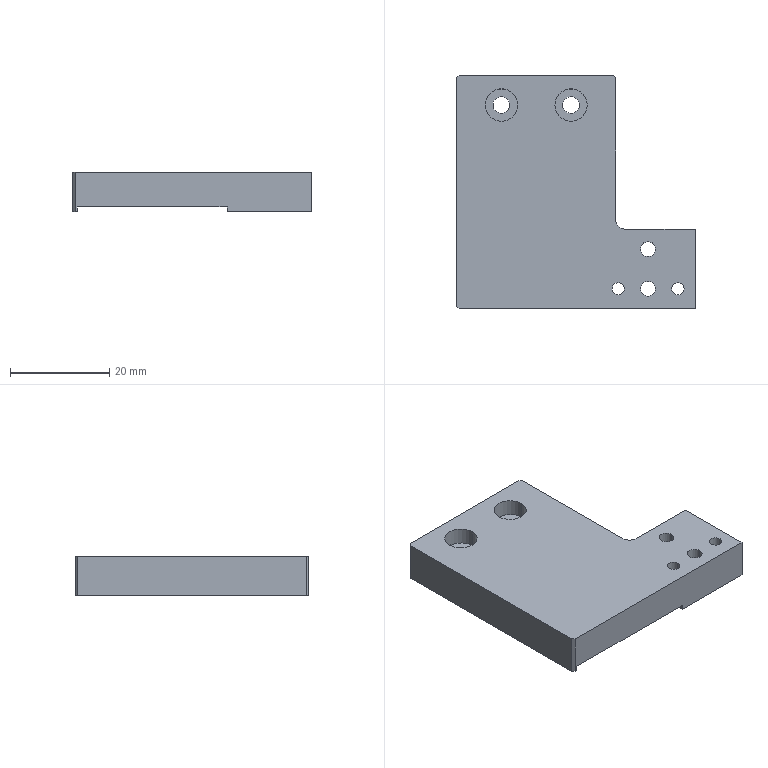Part | STEP file | 11-FG-E03411 | 1 solid | 34 faces | box 48 x 47 x 8 mm | volume 12187 mm3 | cylinder 17 | plane 17 | commonest cylinder face diameters 2.5 x4 3 x4 3.4 x4 6.5 x4 4 x1
STEP:
#1=CARTESIAN_POINT('',(21.005,-11.495,0.));
#2=VERTEX_POINT('',#1);
#3=CARTESIAN_POINT('',(24.005,-11.495,0.));
#4=VERTEX_POINT('',#3);
#5=CARTESIAN_POINT('',(22.505,-11.495,0.));
#6=DIRECTION('',(0.,0.,1.));
#7=DIRECTION('',(1.,0.,0.));
#8=AXIS2_PLACEMENT_3D('',#5,#6,#7);
#9=CIRCLE('',#8,1.5);
#10=EDGE_CURVE('',#2,#4,#9,.T.);
#11=ORIENTED_EDGE('',*,*,#10,.F.);
#12=CARTESIAN_POINT('',(21.005,-11.495,8.));
#13=VERTEX_POINT('',#12);
#14=CARTESIAN_POINT('',(21.005,-11.495,8.));
#15=DIRECTION('',(0.,0.,1.));
#16=VECTOR('',#15,1000.);
#17=LINE('',#14,#16);
#18=EDGE_CURVE('',#2,#13,#17,.T.);
#19=ORIENTED_EDGE('',*,*,#18,.T.);
#20=CARTESIAN_POINT('',(24.005,-11.495,8.));
#21=VERTEX_POINT('',#20);
#22=CARTESIAN_POINT('',(22.505,-11.495,8.));
#23=DIRECTION('',(0.,0.,1.));
#24=DIRECTION('',(1.,0.,0.));
#25=AXIS2_PLACEMENT_3D('',#22,#23,#24);
#26=CIRCLE('',#25,1.5);
#27=EDGE_CURVE('',#13,#21,#26,.T.);
#28=ORIENTED_EDGE('',*,*,#27,.T.);
#29=CARTESIAN_POINT('',(24.005,-11.495,8.));
#30=DIRECTION('',(0.,0.,1.));
#31=VECTOR('',#30,1000.);
#32=LINE('',#29,#31);
#33=EDGE_CURVE('',#4,#21,#32,.T.);
#34=ORIENTED_EDGE('',*,*,#33,.F.);
#35=EDGE_LOOP('',(#11,#19,#28,#34));
#36=FACE_OUTER_BOUND('',#35,.T.);
#37=CARTESIAN_POINT('',(22.505,-11.495,8.));
#38=DIRECTION('',(0.,0.,1.));
#39=DIRECTION('',(1.,0.,0.));
#40=AXIS2_PLACEMENT_3D('',#37,#38,#39);
#41=CYLINDRICAL_SURFACE('',#40,1.5);
#42=ADVANCED_FACE('',(#36),#41,.F.);
#43=CARTESIAN_POINT('',(21.005,-19.495,0.));
#44=VERTEX_POINT('',#43);
#45=CARTESIAN_POINT('',(24.005,-19.495,0.));
#46=VERTEX_POINT('',#45);
#47=CARTESIAN_POINT('',(22.505,-19.495,0.));
#48=DIRECTION('',(0.,0.,1.));
#49=DIRECTION('',(1.,0.,0.));
#50=AXIS2_PLACEMENT_3D('',#47,#48,#49);
#51=CIRCLE('',#50,1.5);
#52=EDGE_CURVE('',#44,#46,#51,.T.);
#53=ORIENTED_EDGE('',*,*,#52,.F.);
#54=CARTESIAN_POINT('',(21.005,-19.495,8.));
#55=VERTEX_POINT('',#54);
#56=CARTESIAN_POINT('',(21.005,-19.495,8.));
#57=DIRECTION('',(0.,0.,1.));
#58=VECTOR('',#57,1000.);
#59=LINE('',#56,#58);
#60=EDGE_CURVE('',#44,#55,#59,.T.);
#61=ORIENTED_EDGE('',*,*,#60,.T.);
#62=CARTESIAN_POINT('',(24.005,-19.495,8.));
#63=VERTEX_POINT('',#62);
#64=CARTESIAN_POINT('',(22.505,-19.495,8.));
#65=DIRECTION('',(0.,0.,1.));
#66=DIRECTION('',(1.,0.,0.));
#67=AXIS2_PLACEMENT_3D('',#64,#65,#66);
#68=CIRCLE('',#67,1.5);
#69=EDGE_CURVE('',#55,#63,#68,.T.);
#70=ORIENTED_EDGE('',*,*,#69,.T.);
#71=CARTESIAN_POINT('',(24.005,-19.495,8.));
#72=DIRECTION('',(0.,0.,1.));
#73=VECTOR('',#72,1000.);
#74=LINE('',#71,#73);
#75=EDGE_CURVE('',#46,#63,#74,.T.);
#76=ORIENTED_EDGE('',*,*,#75,.F.);
#77=EDGE_LOOP('',(#53,#61,#70,#76));
#78=FACE_OUTER_BOUND('',#77,.T.);
#79=CARTESIAN_POINT('',(22.505,-19.495,8.));
#80=DIRECTION('',(0.,0.,1.));
#81=DIRECTION('',(1.,0.,0.));
#82=AXIS2_PLACEMENT_3D('',#79,#80,#81);
#83=CYLINDRICAL_SURFACE('',#82,1.5);
#84=ADVANCED_FACE('',(#78),#83,.F.);
#85=CARTESIAN_POINT('',(27.255,-19.495,0.));
#86=VERTEX_POINT('',#85);
#87=CARTESIAN_POINT('',(29.755,-19.495,0.));
#88=VERTEX_POINT('',#87);
#89=CARTESIAN_POINT('',(28.505,-19.495,0.));
#90=DIRECTION('',(0.,0.,1.));
#91=DIRECTION('',(1.,0.,0.));
#92=AXIS2_PLACEMENT_3D('',#89,#90,#91);
#93=CIRCLE('',#92,1.25);
#94=EDGE_CURVE('',#86,#88,#93,.T.);
#95=ORIENTED_EDGE('',*,*,#94,.F.);
#96=CARTESIAN_POINT('',(27.255,-19.495,8.));
#97=VERTEX_POINT('',#96);
#98=CARTESIAN_POINT('',(27.255,-19.495,8.));
#99=DIRECTION('',(0.,0.,1.));
#100=VECTOR('',#99,1000.);
#101=LINE('',#98,#100);
#102=EDGE_CURVE('',#86,#97,#101,.T.);
#103=ORIENTED_EDGE('',*,*,#102,.T.);
#104=CARTESIAN_POINT('',(29.755,-19.495,8.));
#105=VERTEX_POINT('',#104);
#106=CARTESIAN_POINT('',(28.505,-19.495,8.));
#107=DIRECTION('',(0.,0.,1.));
#108=DIRECTION('',(1.,0.,0.));
#109=AXIS2_PLACEMENT_3D('',#106,#107,#108);
#110=CIRCLE('',#109,1.25);
#111=EDGE_CURVE('',#97,#105,#110,.T.);
#112=ORIENTED_EDGE('',*,*,#111,.T.);
#113=CARTESIAN_POINT('',(29.755,-19.495,8.));
#114=DIRECTION('',(0.,0.,1.));
#115=VECTOR('',#114,1000.);
#116=LINE('',#113,#115);
#117=EDGE_CURVE('',#88,#105,#116,.T.);
#118=ORIENTED_EDGE('',*,*,#117,.F.);
#119=EDGE_LOOP('',(#95,#103,#112,#118));
#120=FACE_OUTER_BOUND('',#119,.T.);
#121=CARTESIAN_POINT('',(28.505,-19.495,8.));
#122=DIRECTION('',(0.,0.,1.));
#123=DIRECTION('',(1.,0.,0.));
#124=AXIS2_PLACEMENT_3D('',#121,#122,#123);
#125=CYLINDRICAL_SURFACE('',#124,1.25);
#126=ADVANCED_FACE('',(#120),#125,.F.);
#127=CARTESIAN_POINT('',(15.255,-19.495,0.));
#128=VERTEX_POINT('',#127);
#129=CARTESIAN_POINT('',(17.755,-19.495,0.));
#130=VERTEX_POINT('',#129);
#131=CARTESIAN_POINT('',(16.505,-19.495,0.));
#132=DIRECTION('',(0.,0.,1.));
#133=DIRECTION('',(1.,0.,0.));
#134=AXIS2_PLACEMENT_3D('',#131,#132,#133);
#135=CIRCLE('',#134,1.25);
#136=EDGE_CURVE('',#128,#130,#135,.T.);
#137=ORIENTED_EDGE('',*,*,#136,.F.);
#138=CARTESIAN_POINT('',(15.255,-19.495,8.));
#139=VERTEX_POINT('',#138);
#140=CARTESIAN_POINT('',(15.255,-19.495,8.));
#141=DIRECTION('',(0.,0.,1.));
#142=VECTOR('',#141,1000.);
#143=LINE('',#140,#142);
#144=EDGE_CURVE('',#128,#139,#143,.T.);
#145=ORIENTED_EDGE('',*,*,#144,.T.);
#146=CARTESIAN_POINT('',(17.755,-19.495,8.));
#147=VERTEX_POINT('',#146);
#148=CARTESIAN_POINT('',(16.505,-19.495,8.));
#149=DIRECTION('',(0.,0.,1.));
#150=DIRECTION('',(1.,0.,0.));
#151=AXIS2_PLACEMENT_3D('',#148,#149,#150);
#152=CIRCLE('',#151,1.25);
#153=EDGE_CURVE('',#139,#147,#152,.T.);
#154=ORIENTED_EDGE('',*,*,#153,.T.);
#155=CARTESIAN_POINT('',(17.755,-19.495,8.));
#156=DIRECTION('',(0.,0.,1.));
#157=VECTOR('',#156,1000.);
#158=LINE('',#155,#157);
#159=EDGE_CURVE('',#130,#147,#158,.T.);
#160=ORIENTED_EDGE('',*,*,#159,.F.);
#161=EDGE_LOOP('',(#137,#145,#154,#160));
#162=FACE_OUTER_BOUND('',#161,.T.);
#163=CARTESIAN_POINT('',(16.505,-19.495,8.));
#164=DIRECTION('',(0.,0.,1.));
#165=DIRECTION('',(1.,0.,0.));
#166=AXIS2_PLACEMENT_3D('',#163,#164,#165);
#167=CYLINDRICAL_SURFACE('',#166,1.25);
#168=ADVANCED_FACE('',(#162),#167,.F.);
#169=CARTESIAN_POINT('',(3.75,17.5,4.6));
#170=VERTEX_POINT('',#169);
#171=CARTESIAN_POINT('',(10.25,17.5,4.6));
#172=VERTEX_POINT('',#171);
#173=CARTESIAN_POINT('',(7.,17.5,4.6));
#174=DIRECTION('',(0.,0.,1.));
#175=DIRECTION('',(1.,0.,0.));
#176=AXIS2_PLACEMENT_3D('',#173,#174,#175);
#177=CIRCLE('',#176,3.25);
#178=EDGE_CURVE('',#170,#172,#177,.T.);
#179=ORIENTED_EDGE('',*,*,#178,.F.);
#180=CARTESIAN_POINT('',(3.75,17.5,8.));
#181=VERTEX_POINT('',#180);
#182=CARTESIAN_POINT('',(3.75,17.5,8.));
#183=DIRECTION('',(0.,0.,1.));
#184=VECTOR('',#183,1000.);
#185=LINE('',#182,#184);
#186=EDGE_CURVE('',#170,#181,#185,.T.);
#187=ORIENTED_EDGE('',*,*,#186,.T.);
#188=CARTESIAN_POINT('',(10.25,17.5,8.));
#189=VERTEX_POINT('',#188);
#190=CARTESIAN_POINT('',(7.,17.5,8.));
#191=DIRECTION('',(0.,0.,1.));
#192=DIRECTION('',(1.,0.,0.));
#193=AXIS2_PLACEMENT_3D('',#190,#191,#192);
#194=CIRCLE('',#193,3.25);
#195=EDGE_CURVE('',#181,#189,#194,.T.);
#196=ORIENTED_EDGE('',*,*,#195,.T.);
#197=CARTESIAN_POINT('',(10.25,17.5,8.));
#198=DIRECTION('',(0.,0.,1.));
#199=VECTOR('',#198,1000.);
#200=LINE('',#197,#199);
#201=EDGE_CURVE('',#172,#189,#200,.T.);
#202=ORIENTED_EDGE('',*,*,#201,.F.);
#203=EDGE_LOOP('',(#179,#187,#196,#202));
#204=FACE_OUTER_BOUND('',#203,.T.);
#205=CARTESIAN_POINT('',(7.,17.5,8.));
#206=DIRECTION('',(0.,0.,1.));
#207=DIRECTION('',(1.,0.,0.));
#208=AXIS2_PLACEMENT_3D('',#205,#206,#207);
#209=CYLINDRICAL_SURFACE('',#208,3.25);
#210=ADVANCED_FACE('',(#204),#209,.F.);
#211=CARTESIAN_POINT('',(5.3,17.5,1.));
#212=VERTEX_POINT('',#211);
#213=CARTESIAN_POINT('',(8.7,17.5,1.));
#214=VERTEX_POINT('',#213);
#215=CARTESIAN_POINT('',(7.,17.5,1.));
#216=DIRECTION('',(0.,0.,1.));
#217=DIRECTION('',(1.,0.,0.));
#218=AXIS2_PLACEMENT_3D('',#215,#216,#217);
#219=CIRCLE('',#218,1.7);
#220=EDGE_CURVE('',#212,#214,#219,.T.);
#221=ORIENTED_EDGE('',*,*,#220,.F.);
#222=CARTESIAN_POINT('',(5.3,17.5,4.6));
#223=VERTEX_POINT('',#222);
#224=CARTESIAN_POINT('',(5.3,17.5,8.));
#225=DIRECTION('',(0.,0.,1.));
#226=VECTOR('',#225,1000.);
#227=LINE('',#224,#226);
#228=EDGE_CURVE('',#212,#223,#227,.T.);
#229=ORIENTED_EDGE('',*,*,#228,.T.);
#230=CARTESIAN_POINT('',(8.7,17.5,4.6));
#231=VERTEX_POINT('',#230);
#232=CARTESIAN_POINT('',(7.,17.5,4.6));
#233=DIRECTION('',(0.,0.,1.));
#234=DIRECTION('',(1.,0.,0.));
#235=AXIS2_PLACEMENT_3D('',#232,#233,#234);
#236=CIRCLE('',#235,1.7);
#237=EDGE_CURVE('',#223,#231,#236,.T.);
#238=ORIENTED_EDGE('',*,*,#237,.T.);
#239=CARTESIAN_POINT('',(8.7,17.5,8.));
#240=DIRECTION('',(0.,0.,1.));
#241=VECTOR('',#240,1000.);
#242=LINE('',#239,#241);
#243=EDGE_CURVE('',#214,#231,#242,.T.);
#244=ORIENTED_EDGE('',*,*,#243,.F.);
#245=EDGE_LOOP('',(#221,#229,#238,#244));
#246=FACE_OUTER_BOUND('',#245,.T.);
#247=CARTESIAN_POINT('',(7.,17.5,8.));
#248=DIRECTION('',(0.,0.,1.));
#249=DIRECTION('',(1.,0.,0.));
#250=AXIS2_PLACEMENT_3D('',#247,#248,#249);
#251=CYLINDRICAL_SURFACE('',#250,1.7);
#252=ADVANCED_FACE('',(#246),#251,.F.);
#253=CARTESIAN_POINT('',(-10.25,17.5,4.6));
#254=VERTEX_POINT('',#253);
#255=CARTESIAN_POINT('',(-3.75,17.5,4.6));
#256=VERTEX_POINT('',#255);
#257=CARTESIAN_POINT('',(-7.,17.5,4.6));
#258=DIRECTION('',(0.,0.,1.));
#259=DIRECTION('',(1.,0.,0.));
#260=AXIS2_PLACEMENT_3D('',#257,#258,#259);
#261=CIRCLE('',#260,3.25);
#262=EDGE_CURVE('',#254,#256,#261,.T.);
#263=ORIENTED_EDGE('',*,*,#262,.F.);
#264=CARTESIAN_POINT('',(-10.25,17.5,8.));
#265=VERTEX_POINT('',#264);
#266=CARTESIAN_POINT('',(-10.25,17.5,8.));
#267=DIRECTION('',(0.,0.,1.));
#268=VECTOR('',#267,1000.);
#269=LINE('',#266,#268);
#270=EDGE_CURVE('',#254,#265,#269,.T.);
#271=ORIENTED_EDGE('',*,*,#270,.T.);
#272=CARTESIAN_POINT('',(-3.75,17.5,8.));
#273=VERTEX_POINT('',#272);
#274=CARTESIAN_POINT('',(-7.,17.5,8.));
#275=DIRECTION('',(0.,0.,1.));
#276=DIRECTION('',(1.,0.,0.));
#277=AXIS2_PLACEMENT_3D('',#274,#275,#276);
#278=CIRCLE('',#277,3.25);
#279=EDGE_CURVE('',#265,#273,#278,.T.);
#280=ORIENTED_EDGE('',*,*,#279,.T.);
#281=CARTESIAN_POINT('',(-3.75,17.5,8.));
#282=DIRECTION('',(0.,0.,1.));
#283=VECTOR('',#282,1000.);
#284=LINE('',#281,#283);
#285=EDGE_CURVE('',#256,#273,#284,.T.);
#286=ORIENTED_EDGE('',*,*,#285,.F.);
#287=EDGE_LOOP('',(#263,#271,#280,#286));
#288=FACE_OUTER_BOUND('',#287,.T.);
#289=CARTESIAN_POINT('',(-7.,17.5,8.));
#290=DIRECTION('',(0.,0.,1.));
#291=DIRECTION('',(1.,0.,0.));
#292=AXIS2_PLACEMENT_3D('',#289,#290,#291);
#293=CYLINDRICAL_SURFACE('',#292,3.25);
#294=ADVANCED_FACE('',(#288),#293,.F.);
#295=CARTESIAN_POINT('',(-8.7,17.5,1.));
#296=VERTEX_POINT('',#295);
#297=CARTESIAN_POINT('',(-5.3,17.5,1.));
#298=VERTEX_POINT('',#297);
#299=CARTESIAN_POINT('',(-7.,17.5,1.));
#300=DIRECTION('',(0.,0.,1.));
#301=DIRECTION('',(1.,0.,0.));
#302=AXIS2_PLACEMENT_3D('',#299,#300,#301);
#303=CIRCLE('',#302,1.7);
#304=EDGE_CURVE('',#296,#298,#303,.T.);
#305=ORIENTED_EDGE('',*,*,#304,.F.);
#306=CARTESIAN_POINT('',(-8.7,17.5,4.6));
#307=VERTEX_POINT('',#306);
#308=CARTESIAN_POINT('',(-8.7,17.5,8.));
#309=DIRECTION('',(0.,0.,1.));
#310=VECTOR('',#309,1000.);
#311=LINE('',#308,#310);
#312=EDGE_CURVE('',#296,#307,#311,.T.);
#313=ORIENTED_EDGE('',*,*,#312,.T.);
#314=CARTESIAN_POINT('',(-5.3,17.5,4.6));
#315=VERTEX_POINT('',#314);
#316=CARTESIAN_POINT('',(-7.,17.5,4.6));
#317=DIRECTION('',(0.,0.,1.));
#318=DIRECTION('',(1.,0.,0.));
#319=AXIS2_PLACEMENT_3D('',#316,#317,#318);
#320=CIRCLE('',#319,1.7);
#321=EDGE_CURVE('',#307,#315,#320,.T.);
#322=ORIENTED_EDGE('',*,*,#321,.T.);
#323=CARTESIAN_POINT('',(-5.3,17.5,8.));
#324=DIRECTION('',(0.,0.,1.));
#325=VECTOR('',#324,1000.);
#326=LINE('',#323,#325);
#327=EDGE_CURVE('',#298,#315,#326,.T.);
#328=ORIENTED_EDGE('',*,*,#327,.F.);
#329=EDGE_LOOP('',(#305,#313,#322,#328));
#330=FACE_OUTER_BOUND('',#329,.T.);
#331=CARTESIAN_POINT('',(-7.,17.5,8.));
#332=DIRECTION('',(0.,0.,1.));
#333=DIRECTION('',(1.,0.,0.));
#334=AXIS2_PLACEMENT_3D('',#331,#332,#333);
#335=CYLINDRICAL_SURFACE('',#334,1.7);
#336=ADVANCED_FACE('',(#330),#335,.F.);
#337=CARTESIAN_POINT('',(16.,-5.5,8.));
#338=VERTEX_POINT('',#337);
#339=CARTESIAN_POINT('',(16.,23.,8.));
#340=VERTEX_POINT('',#339);
#341=CARTESIAN_POINT('',(16.,-23.5,8.));
#342=DIRECTION('',(0.,1.,0.));
#343=VECTOR('',#342,1000.);
#344=LINE('',#341,#343);
#345=EDGE_CURVE('',#338,#340,#344,.T.);
#346=ORIENTED_EDGE('',*,*,#345,.F.);
#347=CARTESIAN_POINT('',(16.,-5.5,0.));
#348=VERTEX_POINT('',#347);
#349=CARTESIAN_POINT('',(16.,-5.5,8.));
#350=DIRECTION('',(0.,0.,-1.));
#351=VECTOR('',#350,1000.);
#352=LINE('',#349,#351);
#353=EDGE_CURVE('',#338,#348,#352,.T.);
#354=ORIENTED_EDGE('',*,*,#353,.T.);
#355=CARTESIAN_POINT('',(16.,23.,0.));
#356=VERTEX_POINT('',#355);
#357=CARTESIAN_POINT('',(16.,-23.5,0.));
#358=DIRECTION('',(0.,1.,0.));
#359=VECTOR('',#358,1000.);
#360=LINE('',#357,#359);
#361=EDGE_CURVE('',#348,#356,#360,.T.);
#362=ORIENTED_EDGE('',*,*,#361,.T.);
#363=CARTESIAN_POINT('',(16.,23.,8.));
#364=DIRECTION('',(0.,0.,1.));
#365=VECTOR('',#364,1000.);
#366=LINE('',#363,#365);
#367=EDGE_CURVE('',#356,#340,#366,.T.);
#368=ORIENTED_EDGE('',*,*,#367,.T.);
#369=EDGE_LOOP('',(#346,#354,#362,#368));
#370=FACE_OUTER_BOUND('',#369,.T.);
#371=CARTESIAN_POINT('',(16.,-23.5,8.));
#372=DIRECTION('',(-1.,0.,0.));
#373=DIRECTION('',(0.,0.,1.));
#374=AXIS2_PLACEMENT_3D('',#371,#372,#373);
#375=PLANE('',#374);
#376=ADVANCED_FACE('',(#370),#375,.F.);
#377=CARTESIAN_POINT('',(22.505,-11.495,0.));
#378=DIRECTION('',(0.,0.,1.));
#379=DIRECTION('',(1.,0.,0.));
#380=AXIS2_PLACEMENT_3D('',#377,#378,#379);
#381=CIRCLE('',#380,1.5);
#382=EDGE_CURVE('',#4,#2,#381,.T.);
#383=ORIENTED_EDGE('',*,*,#382,.T.);
#384=ORIENTED_EDGE('',*,*,#10,.T.);
#385=EDGE_LOOP('',(#383,#384));
#386=FACE_BOUND('',#385,.T.);
#387=CARTESIAN_POINT('',(22.505,-19.495,0.));
#388=DIRECTION('',(0.,0.,1.));
#389=DIRECTION('',(1.,0.,0.));
#390=AXIS2_PLACEMENT_3D('',#387,#388,#389);
#391=CIRCLE('',#390,1.5);
#392=EDGE_CURVE('',#46,#44,#391,.T.);
#393=ORIENTED_EDGE('',*,*,#392,.T.);
#394=ORIENTED_EDGE('',*,*,#52,.T.);
#395=EDGE_LOOP('',(#393,#394));
#396=FACE_BOUND('',#395,.T.);
#397=CARTESIAN_POINT('',(28.505,-19.495,0.));
#398=DIRECTION('',(0.,0.,1.));
#399=DIRECTION('',(1.,0.,0.));
#400=AXIS2_PLACEMENT_3D('',#397,#398,#399);
#401=CIRCLE('',#400,1.25);
#402=EDGE_CURVE('',#88,#86,#401,.T.);
#403=ORIENTED_EDGE('',*,*,#402,.T.);
#404=ORIENTED_EDGE('',*,*,#94,.T.);
#405=EDGE_LOOP('',(#403,#404));
#406=FACE_BOUND('',#405,.T.);
#407=CARTESIAN_POINT('',(16.505,-19.495,0.));
#408=DIRECTION('',(0.,0.,1.));
#409=DIRECTION('',(1.,0.,0.));
#410=AXIS2_PLACEMENT_3D('',#407,#408,#409);
#411=CIRCLE('',#410,1.25);
#412=EDGE_CURVE('',#130,#128,#411,.T.);
#413=ORIENTED_EDGE('',*,*,#412,.T.);
#414=ORIENTED_EDGE('',*,*,#136,.T.);
#415=EDGE_LOOP('',(#413,#414));
#416=FACE_BOUND('',#415,.T.);
#417=CARTESIAN_POINT('',(15.5,23.5,0.));
#418=VERTEX_POINT('',#417);
#419=CARTESIAN_POINT('',(15.05,23.5,0.));
#420=VERTEX_POINT('',#419);
#421=CARTESIAN_POINT('',(-16.,23.5,0.));
#422=DIRECTION('',(-1.,0.,0.));
#423=VECTOR('',#422,1000.);
#424=LINE('',#421,#423);
#425=EDGE_CURVE('',#418,#420,#424,.T.);
#426=ORIENTED_EDGE('',*,*,#425,.F.);
#427=CARTESIAN_POINT('',(19.5,19.5,0.));
#428=DIRECTION('',(0.7071,-0.7071,0.));
#429=VECTOR('',#428,1000.);
#430=LINE('',#427,#429);
#431=EDGE_CURVE('',#418,#356,#430,.T.);
#432=ORIENTED_EDGE('',*,*,#431,.T.);
#433=ORIENTED_EDGE('',*,*,#361,.F.);
#434=CARTESIAN_POINT('',(18.,-7.5,0.));
#435=VERTEX_POINT('',#434);
#436=CARTESIAN_POINT('',(18.,-5.5,0.));
#437=DIRECTION('',(0.,0.,1.));
#438=DIRECTION('',(-1.,0.,0.));
#439=AXIS2_PLACEMENT_3D('',#436,#437,#438);
#440=CIRCLE('',#439,2.);
#441=EDGE_CURVE('',#348,#435,#440,.T.);
#442=ORIENTED_EDGE('',*,*,#441,.T.);
#443=CARTESIAN_POINT('',(32.,-7.5,0.));
#444=VERTEX_POINT('',#443);
#445=CARTESIAN_POINT('',(16.,-7.5,0.));
#446=DIRECTION('',(-1.,0.,0.));
#447=VECTOR('',#446,1000.);
#448=LINE('',#445,#447);
#449=EDGE_CURVE('',#444,#435,#448,.T.);
#450=ORIENTED_EDGE('',*,*,#449,.F.);
#451=CARTESIAN_POINT('',(32.,-23.5,0.));
#452=VERTEX_POINT('',#451);
#453=CARTESIAN_POINT('',(32.,-23.5,0.));
#454=DIRECTION('',(0.,1.,0.));
#455=VECTOR('',#454,1000.);
#456=LINE('',#453,#455);
#457=EDGE_CURVE('',#452,#444,#456,.T.);
#458=ORIENTED_EDGE('',*,*,#457,.F.);
#459=CARTESIAN_POINT('',(15.05,-23.5,0.));
#460=VERTEX_POINT('',#459);
#461=CARTESIAN_POINT('',(-16.,-23.5,0.));
#462=DIRECTION('',(1.,0.,0.));
#463=VECTOR('',#462,1000.);
#464=LINE('',#461,#463);
#465=EDGE_CURVE('',#460,#452,#464,.T.);
#466=ORIENTED_EDGE('',*,*,#465,.F.);
#467=CARTESIAN_POINT('',(15.05,0.,0.));
#468=DIRECTION('',(0.,-1.,0.));
#469=VECTOR('',#468,1000.);
#470=LINE('',#467,#469);
#471=EDGE_CURVE('',#420,#460,#470,.T.);
#472=ORIENTED_EDGE('',*,*,#471,.F.);
#473=EDGE_LOOP('',(#426,#432,#433,#442,#450,#458,#466,#472));
#474=FACE_OUTER_BOUND('',#473,.T.);
#475=CARTESIAN_POINT('',(0.,0.,0.));
#476=DIRECTION('',(0.,0.,-1.));
#477=DIRECTION('',(-1.,0.,0.));
#478=AXIS2_PLACEMENT_3D('',#475,#476,#477);
#479=PLANE('',#478);
#480=ADVANCED_FACE('',(#386,#396,#406,#416,#474),#479,.T.);
#481=CARTESIAN_POINT('',(-15.05,23.5,0.));
#482=VERTEX_POINT('',#481);
#483=CARTESIAN_POINT('',(-15.5,23.5,0.));
#484=VERTEX_POINT('',#483);
#485=CARTESIAN_POINT('',(-16.,23.5,0.));
#486=DIRECTION('',(-1.,0.,0.));
#487=VECTOR('',#486,1000.);
#488=LINE('',#485,#487);
#489=EDGE_CURVE('',#482,#484,#488,.T.);
#490=ORIENTED_EDGE('',*,*,#489,.T.);
#491=CARTESIAN_POINT('',(-15.5,23.5,8.));
#492=VERTEX_POINT('',#491);
#493=CARTESIAN_POINT('',(-15.5,23.5,8.));
#494=DIRECTION('',(0.,0.,1.));
#495=VECTOR('',#494,1000.);
#496=LINE('',#493,#495);
#497=EDGE_CURVE('',#484,#492,#496,.T.);
#498=ORIENTED_EDGE('',*,*,#497,.T.);
#499=CARTESIAN_POINT('',(15.5,23.5,8.));
#500=VERTEX_POINT('',#499);
#501=CARTESIAN_POINT('',(-16.,23.5,8.));
#502=DIRECTION('',(-1.,0.,0.));
#503=VECTOR('',#502,1000.);
#504=LINE('',#501,#503);
#505=EDGE_CURVE('',#500,#492,#504,.T.);
#506=ORIENTED_EDGE('',*,*,#505,.F.);
#507=CARTESIAN_POINT('',(15.5,23.5,8.));
#508=DIRECTION('',(0.,0.,-1.));
#509=VECTOR('',#508,1000.);
#510=LINE('',#507,#509);
#511=EDGE_CURVE('',#500,#418,#510,.T.);
#512=ORIENTED_EDGE('',*,*,#511,.T.);
#513=ORIENTED_EDGE('',*,*,#425,.T.);
#514=CARTESIAN_POINT('',(15.05,23.5,1.));
#515=VERTEX_POINT('',#514);
#516=CARTESIAN_POINT('',(15.05,23.5,1.));
#517=DIRECTION('',(0.,0.,-1.));
#518=VECTOR('',#517,1000.);
#519=LINE('',#516,#518);
#520=EDGE_CURVE('',#515,#420,#519,.T.);
#521=ORIENTED_EDGE('',*,*,#520,.F.);
#522=CARTESIAN_POINT('',(-15.05,23.5,1.));
#523=VERTEX_POINT('',#522);
#524=CARTESIAN_POINT('',(15.05,23.5,1.));
#525=DIRECTION('',(1.,0.,0.));
#526=VECTOR('',#525,1000.);
#527=LINE('',#524,#526);
#528=EDGE_CURVE('',#523,#515,#527,.T.);
#529=ORIENTED_EDGE('',*,*,#528,.F.);
#530=CARTESIAN_POINT('',(-15.05,23.5,1.));
#531=DIRECTION('',(0.,0.,1.));
#532=VECTOR('',#531,1000.);
#533=LINE('',#530,#532);
#534=EDGE_CURVE('',#482,#523,#533,.T.);
#535=ORIENTED_EDGE('',*,*,#534,.F.);
#536=EDGE_LOOP('',(#490,#498,#506,#512,#513,#521,#529,#535));
#537=FACE_OUTER_BOUND('',#536,.T.);
#538=CARTESIAN_POINT('',(-16.,23.5,8.));
#539=DIRECTION('',(0.,-1.,0.));
#540=DIRECTION('',(0.,0.,-1.));
#541=AXIS2_PLACEMENT_3D('',#538,#539,#540);
#542=PLANE('',#541);
#543=ADVANCED_FACE('',(#537),#542,.F.);
#544=CARTESIAN_POINT('',(-16.,23.,8.));
#545=VERTEX_POINT('',#544);
#546=CARTESIAN_POINT('',(-16.,-23.,8.));
#547=VERTEX_POINT('',#546);
#548=CARTESIAN_POINT('',(-16.,-23.5,8.));
#549=DIRECTION('',(0.,-1.,0.));
#550=VECTOR('',#549,1000.);
#551=LINE('',#548,#550);
#552=EDGE_CURVE('',#545,#547,#551,.T.);
#553=ORIENTED_EDGE('',*,*,#552,.F.);
#554=CARTESIAN_POINT('',(-16.,23.,0.));
#555=VERTEX_POINT('',#554);
#556=CARTESIAN_POINT('',(-16.,23.,8.));
#557=DIRECTION('',(0.,0.,-1.));
#558=VECTOR('',#557,1000.);
#559=LINE('',#556,#558);
#560=EDGE_CURVE('',#545,#555,#559,.T.);
#561=ORIENTED_EDGE('',*,*,#560,.T.);
#562=CARTESIAN_POINT('',(-16.,-23.,0.));
#563=VERTEX_POINT('',#562);
#564=CARTESIAN_POINT('',(-16.,-23.5,0.));
#565=DIRECTION('',(0.,-1.,0.));
#566=VECTOR('',#565,1000.);
#567=LINE('',#564,#566);
#568=EDGE_CURVE('',#555,#563,#567,.T.);
#569=ORIENTED_EDGE('',*,*,#568,.T.);
#570=CARTESIAN_POINT('',(-16.,-23.,8.));
#571=DIRECTION('',(0.,0.,1.));
#572=VECTOR('',#571,1000.);
#573=LINE('',#570,#572);
#574=EDGE_CURVE('',#563,#547,#573,.T.);
#575=ORIENTED_EDGE('',*,*,#574,.T.);
#576=EDGE_LOOP('',(#553,#561,#569,#575));
#577=FACE_OUTER_BOUND('',#576,.T.);
#578=CARTESIAN_POINT('',(-16.,-23.5,8.));
#579=DIRECTION('',(1.,0.,0.));
#580=DIRECTION('',(0.,0.,-1.));
#581=AXIS2_PLACEMENT_3D('',#578,#579,#580);
#582=PLANE('',#581);
#583=ADVANCED_FACE('',(#577),#582,.F.);
#584=CARTESIAN_POINT('',(-15.5,-23.5,8.));
#585=VERTEX_POINT('',#584);
#586=CARTESIAN_POINT('',(32.,-23.5,8.));
#587=VERTEX_POINT('',#586);
#588=CARTESIAN_POINT('',(-16.,-23.5,8.));
#589=DIRECTION('',(1.,0.,0.));
#590=VECTOR('',#589,1000.);
#591=LINE('',#588,#590);
#592=EDGE_CURVE('',#585,#587,#591,.T.);
#593=ORIENTED_EDGE('',*,*,#592,.F.);
#594=CARTESIAN_POINT('',(-15.5,-23.5,0.));
#595=VERTEX_POINT('',#594);
#596=CARTESIAN_POINT('',(-15.5,-23.5,8.));
#597=DIRECTION('',(0.,0.,-1.));
#598=VECTOR('',#597,1000.);
#599=LINE('',#596,#598);
#600=EDGE_CURVE('',#585,#595,#599,.T.);
#601=ORIENTED_EDGE('',*,*,#600,.T.);
#602=CARTESIAN_POINT('',(-15.05,-23.5,0.));
#603=VERTEX_POINT('',#602);
#604=CARTESIAN_POINT('',(-16.,-23.5,0.));
#605=DIRECTION('',(1.,0.,0.));
#606=VECTOR('',#605,1000.);
#607=LINE('',#604,#606);
#608=EDGE_CURVE('',#595,#603,#607,.T.);
#609=ORIENTED_EDGE('',*,*,#608,.T.);
#610=CARTESIAN_POINT('',(-15.05,-23.5,1.));
#611=VERTEX_POINT('',#610);
#612=CARTESIAN_POINT('',(-15.05,-23.5,8.));
#613=DIRECTION('',(0.,0.,1.));
#614=VECTOR('',#613,1000.);
#615=LINE('',#612,#614);
#616=EDGE_CURVE('',#603,#611,#615,.T.);
#617=ORIENTED_EDGE('',*,*,#616,.T.);
#618=CARTESIAN_POINT('',(15.05,-23.5,1.));
#619=VERTEX_POINT('',#618);
#620=CARTESIAN_POINT('',(-16.,-23.5,1.));
#621=DIRECTION('',(1.,0.,0.));
#622=VECTOR('',#621,1000.);
#623=LINE('',#620,#622);
#624=EDGE_CURVE('',#611,#619,#623,.T.);
#625=ORIENTED_EDGE('',*,*,#624,.T.);
#626=CARTESIAN_POINT('',(15.05,-23.5,8.));
#627=DIRECTION('',(0.,0.,-1.));
#628=VECTOR('',#627,1000.);
#629=LINE('',#626,#628);
#630=EDGE_CURVE('',#619,#460,#629,.T.);
#631=ORIENTED_EDGE('',*,*,#630,.T.);
#632=ORIENTED_EDGE('',*,*,#465,.T.);
#633=CARTESIAN_POINT('',(32.,-23.5,-22.627));
#634=DIRECTION('',(0.,0.,1.));
#635=VECTOR('',#634,1000.);
#636=LINE('',#633,#635);
#637=EDGE_CURVE('',#452,#587,#636,.T.);
#638=ORIENTED_EDGE('',*,*,#637,.T.);
#639=EDGE_LOOP('',(#593,#601,#609,#617,#625,#631,#632,#638));
#640=FACE_OUTER_BOUND('',#639,.T.);
#641=CARTESIAN_POINT('',(-16.,-23.5,8.));
#642=DIRECTION('',(0.,1.,0.));
#643=DIRECTION('',(0.,0.,1.));
#644=AXIS2_PLACEMENT_3D('',#641,#642,#643);
#645=PLANE('',#644);
#646=ADVANCED_FACE('',(#640),#645,.F.);
#647=CARTESIAN_POINT('',(22.505,-11.495,8.));
#648=DIRECTION('',(0.,0.,1.));
#649=DIRECTION('',(1.,0.,0.));
#650=AXIS2_PLACEMENT_3D('',#647,#648,#649);
#651=CIRCLE('',#650,1.5);
#652=EDGE_CURVE('',#21,#13,#651,.T.);
#653=ORIENTED_EDGE('',*,*,#652,.F.);
#654=ORIENTED_EDGE('',*,*,#27,.F.);
#655=EDGE_LOOP('',(#653,#654));
#656=FACE_BOUND('',#655,.T.);
#657=CARTESIAN_POINT('',(22.505,-19.495,8.));
#658=DIRECTION('',(0.,0.,1.));
#659=DIRECTION('',(1.,0.,0.));
#660=AXIS2_PLACEMENT_3D('',#657,#658,#659);
#661=CIRCLE('',#660,1.5);
#662=EDGE_CURVE('',#63,#55,#661,.T.);
#663=ORIENTED_EDGE('',*,*,#662,.F.);
#664=ORIENTED_EDGE('',*,*,#69,.F.);
#665=EDGE_LOOP('',(#663,#664));
#666=FACE_BOUND('',#665,.T.);
#667=CARTESIAN_POINT('',(28.505,-19.495,8.));
#668=DIRECTION('',(0.,0.,1.));
#669=DIRECTION('',(1.,0.,0.));
#670=AXIS2_PLACEMENT_3D('',#667,#668,#669);
#671=CIRCLE('',#670,1.25);
#672=EDGE_CURVE('',#105,#97,#671,.T.);
#673=ORIENTED_EDGE('',*,*,#672,.F.);
#674=ORIENTED_EDGE('',*,*,#111,.F.);
#675=EDGE_LOOP('',(#673,#674));
#676=FACE_BOUND('',#675,.T.);
#677=CARTESIAN_POINT('',(16.505,-19.495,8.));
#678=DIRECTION('',(0.,0.,1.));
#679=DIRECTION('',(1.,0.,0.));
#680=AXIS2_PLACEMENT_3D('',#677,#678,#679);
#681=CIRCLE('',#680,1.25);
#682=EDGE_CURVE('',#147,#139,#681,.T.);
#683=ORIENTED_EDGE('',*,*,#682,.F.);
#684=ORIENTED_EDGE('',*,*,#153,.F.);
#685=EDGE_LOOP('',(#683,#684));
#686=FACE_BOUND('',#685,.T.);
#687=CARTESIAN_POINT('',(7.,17.5,8.));
#688=DIRECTION('',(0.,0.,1.));
#689=DIRECTION('',(1.,0.,0.));
#690=AXIS2_PLACEMENT_3D('',#687,#688,#689);
#691=CIRCLE('',#690,3.25);
#692=EDGE_CURVE('',#189,#181,#691,.T.);
#693=ORIENTED_EDGE('',*,*,#692,.F.);
#694=ORIENTED_EDGE('',*,*,#195,.F.);
#695=EDGE_LOOP('',(#693,#694));
#696=FACE_BOUND('',#695,.T.);
#697=CARTESIAN_POINT('',(-7.,17.5,8.));
#698=DIRECTION('',(0.,0.,1.));
#699=DIRECTION('',(1.,0.,0.));
#700=AXIS2_PLACEMENT_3D('',#697,#698,#699);
#701=CIRCLE('',#700,3.25);
#702=EDGE_CURVE('',#273,#265,#701,.T.);
#703=ORIENTED_EDGE('',*,*,#702,.F.);
#704=ORIENTED_EDGE('',*,*,#279,.F.);
#705=EDGE_LOOP('',(#703,#704));
#706=FACE_BOUND('',#705,.T.);
#707=ORIENTED_EDGE('',*,*,#505,.T.);
#708=CARTESIAN_POINT('',(-16.,23.,8.));
#709=DIRECTION('',(-0.7071,-0.7071,0.));
#710=VECTOR('',#709,1000.);
#711=LINE('',#708,#710);
#712=EDGE_CURVE('',#492,#545,#711,.T.);
#713=ORIENTED_EDGE('',*,*,#712,.T.);
#714=ORIENTED_EDGE('',*,*,#552,.T.);
#715=CARTESIAN_POINT('',(-15.5,-23.5,8.));
#716=DIRECTION('',(0.7071,-0.7071,0.));
#717=VECTOR('',#716,1000.);
#718=LINE('',#715,#717);
#719=EDGE_CURVE('',#547,#585,#718,.T.);
#720=ORIENTED_EDGE('',*,*,#719,.T.);
#721=ORIENTED_EDGE('',*,*,#592,.T.);
#722=CARTESIAN_POINT('',(32.,-7.5,8.));
#723=VERTEX_POINT('',#722);
#724=CARTESIAN_POINT('',(32.,-23.5,8.));
#725=DIRECTION('',(0.,1.,0.));
#726=VECTOR('',#725,1000.);
#727=LINE('',#724,#726);
#728=EDGE_CURVE('',#587,#723,#727,.T.);
#729=ORIENTED_EDGE('',*,*,#728,.T.);
#730=CARTESIAN_POINT('',(18.,-7.5,8.));
#731=VERTEX_POINT('',#730);
#732=CARTESIAN_POINT('',(16.,-7.5,8.));
#733=DIRECTION('',(-1.,0.,0.));
#734=VECTOR('',#733,1000.);
#735=LINE('',#732,#734);
#736=EDGE_CURVE('',#723,#731,#735,.T.);
#737=ORIENTED_EDGE('',*,*,#736,.T.);
#738=CARTESIAN_POINT('',(18.,-5.5,8.));
#739=DIRECTION('',(0.,0.,-1.));
#740=DIRECTION('',(-1.,0.,0.));
#741=AXIS2_PLACEMENT_3D('',#738,#739,#740);
#742=CIRCLE('',#741,2.);
#743=EDGE_CURVE('',#731,#338,#742,.T.);
#744=ORIENTED_EDGE('',*,*,#743,.T.);
#745=ORIENTED_EDGE('',*,*,#345,.T.);
#746=CARTESIAN_POINT('',(15.5,23.5,8.));
#747=DIRECTION('',(-0.7071,0.7071,0.));
#748=VECTOR('',#747,1000.);
#749=LINE('',#746,#748);
#750=EDGE_CURVE('',#340,#500,#749,.T.);
#751=ORIENTED_EDGE('',*,*,#750,.T.);
#752=EDGE_LOOP('',(#707,#713,#714,#720,#721,#729,#737,#744,#745,#751));
#753=FACE_OUTER_BOUND('',#752,.T.);
#754=CARTESIAN_POINT('',(0.,0.,8.));
#755=DIRECTION('',(0.,0.,-1.));
#756=DIRECTION('',(-1.,0.,0.));
#757=AXIS2_PLACEMENT_3D('',#754,#755,#756);
#758=PLANE('',#757);
#759=ADVANCED_FACE('',(#656,#666,#676,#686,#696,#706,#753),#758,.F.);
#760=ORIENTED_EDGE('',*,*,#568,.F.);
#761=CARTESIAN_POINT('',(-19.5,19.5,0.));
#762=DIRECTION('',(0.7071,0.7071,0.));
#763=VECTOR('',#762,1000.);
#764=LINE('',#761,#763);
#765=EDGE_CURVE('',#555,#484,#764,.T.);
#766=ORIENTED_EDGE('',*,*,#765,.T.);
#767=ORIENTED_EDGE('',*,*,#489,.F.);
#768=CARTESIAN_POINT('',(-15.05,0.,0.));
#769=DIRECTION('',(0.,1.,0.));
#770=VECTOR('',#769,1000.);
#771=LINE('',#768,#770);
#772=EDGE_CURVE('',#603,#482,#771,.T.);
#773=ORIENTED_EDGE('',*,*,#772,.F.);
#774=ORIENTED_EDGE('',*,*,#608,.F.);
#775=CARTESIAN_POINT('',(-19.5,-19.5,0.));
#776=DIRECTION('',(-0.7071,0.7071,0.));
#777=VECTOR('',#776,1000.);
#778=LINE('',#775,#777);
#779=EDGE_CURVE('',#595,#563,#778,.T.);
#780=ORIENTED_EDGE('',*,*,#779,.T.);
#781=EDGE_LOOP('',(#760,#766,#767,#773,#774,#780));
#782=FACE_OUTER_BOUND('',#781,.T.);
#783=CARTESIAN_POINT('',(0.,0.,0.));
#784=DIRECTION('',(0.,0.,-1.));
#785=DIRECTION('',(-1.,0.,0.));
#786=AXIS2_PLACEMENT_3D('',#783,#784,#785);
#787=PLANE('',#786);
#788=ADVANCED_FACE('',(#782),#787,.T.);
#789=CARTESIAN_POINT('',(7.,17.5,1.));
#790=DIRECTION('',(0.,0.,1.));
#791=DIRECTION('',(1.,0.,0.));
#792=AXIS2_PLACEMENT_3D('',#789,#790,#791);
#793=CIRCLE('',#792,1.7);
#794=EDGE_CURVE('',#214,#212,#793,.T.);
#795=ORIENTED_EDGE('',*,*,#794,.T.);
#796=ORIENTED_EDGE('',*,*,#220,.T.);
#797=EDGE_LOOP('',(#795,#796));
#798=FACE_BOUND('',#797,.T.);
#799=CARTESIAN_POINT('',(-7.,17.5,1.));
#800=DIRECTION('',(0.,0.,1.));
#801=DIRECTION('',(1.,0.,0.));
#802=AXIS2_PLACEMENT_3D('',#799,#800,#801);
#803=CIRCLE('',#802,1.7);
#804=EDGE_CURVE('',#298,#296,#803,.T.);
#805=ORIENTED_EDGE('',*,*,#804,.T.);
#806=ORIENTED_EDGE('',*,*,#304,.T.);
#807=EDGE_LOOP('',(#805,#806));
#808=FACE_BOUND('',#807,.T.);
#809=CARTESIAN_POINT('',(-15.05,-32.5,1.));
#810=DIRECTION('',(0.,1.,0.));
#811=VECTOR('',#810,1000.);
#812=LINE('',#809,#811);
#813=EDGE_CURVE('',#611,#523,#812,.T.);
#814=ORIENTED_EDGE('',*,*,#813,.T.);
#815=ORIENTED_EDGE('',*,*,#528,.T.);
#816=CARTESIAN_POINT('',(15.05,-32.5,1.));
#817=DIRECTION('',(0.,1.,0.));
#818=VECTOR('',#817,1000.);
#819=LINE('',#816,#818);
#820=EDGE_CURVE('',#619,#515,#819,.T.);
#821=ORIENTED_EDGE('',*,*,#820,.F.);
#822=ORIENTED_EDGE('',*,*,#624,.F.);
#823=EDGE_LOOP('',(#814,#815,#821,#822));
#824=FACE_OUTER_BOUND('',#823,.T.);
#825=CARTESIAN_POINT('',(15.05,-32.5,1.));
#826=DIRECTION('',(0.,0.,1.));
#827=DIRECTION('',(1.,0.,0.));
#828=AXIS2_PLACEMENT_3D('',#825,#826,#827);
#829=PLANE('',#828);
#830=ADVANCED_FACE('',(#798,#808,#824),#829,.F.);
#831=ORIENTED_EDGE('',*,*,#820,.T.);
#832=ORIENTED_EDGE('',*,*,#520,.T.);
#833=ORIENTED_EDGE('',*,*,#471,.T.);
#834=ORIENTED_EDGE('',*,*,#630,.F.);
#835=EDGE_LOOP('',(#831,#832,#833,#834));
#836=FACE_OUTER_BOUND('',#835,.T.);
#837=CARTESIAN_POINT('',(15.05,-32.5,1.));
#838=DIRECTION('',(1.,0.,0.));
#839=DIRECTION('',(0.,0.,-1.));
#840=AXIS2_PLACEMENT_3D('',#837,#838,#839);
#841=PLANE('',#840);
#842=ADVANCED_FACE('',(#836),#841,.F.);
#843=ORIENTED_EDGE('',*,*,#772,.T.);
#844=ORIENTED_EDGE('',*,*,#534,.T.);
#845=ORIENTED_EDGE('',*,*,#813,.F.);
#846=ORIENTED_EDGE('',*,*,#616,.F.);
#847=EDGE_LOOP('',(#843,#844,#845,#846));
#848=FACE_OUTER_BOUND('',#847,.T.);
#849=CARTESIAN_POINT('',(-15.05,-32.5,1.));
#850=DIRECTION('',(-1.,0.,0.));
#851=DIRECTION('',(0.,0.,1.));
#852=AXIS2_PLACEMENT_3D('',#849,#850,#851);
#853=PLANE('',#852);
#854=ADVANCED_FACE('',(#848),#853,.F.);
#855=ORIENTED_EDGE('',*,*,#312,.F.);
#856=ORIENTED_EDGE('',*,*,#804,.F.);
#857=ORIENTED_EDGE('',*,*,#327,.T.);
#858=CARTESIAN_POINT('',(-7.,17.5,4.6));
#859=DIRECTION('',(0.,0.,1.));
#860=DIRECTION('',(1.,0.,0.));
#861=AXIS2_PLACEMENT_3D('',#858,#859,#860);
#862=CIRCLE('',#861,1.7);
#863=EDGE_CURVE('',#315,#307,#862,.T.);
#864=ORIENTED_EDGE('',*,*,#863,.T.);
#865=EDGE_LOOP('',(#855,#856,#857,#864));
#866=FACE_OUTER_BOUND('',#865,.T.);
#867=CARTESIAN_POINT('',(-7.,17.5,8.));
#868=DIRECTION('',(0.,0.,1.));
#869=DIRECTION('',(1.,0.,0.));
#870=AXIS2_PLACEMENT_3D('',#867,#868,#869);
#871=CYLINDRICAL_SURFACE('',#870,1.7);
#872=ADVANCED_FACE('',(#866),#871,.F.);
#873=ORIENTED_EDGE('',*,*,#863,.F.);
#874=ORIENTED_EDGE('',*,*,#321,.F.);
#875=EDGE_LOOP('',(#873,#874));
#876=FACE_BOUND('',#875,.T.);
#877=CARTESIAN_POINT('',(-7.,17.5,4.6));
#878=DIRECTION('',(0.,0.,1.));
#879=DIRECTION('',(1.,0.,0.));
#880=AXIS2_PLACEMENT_3D('',#877,#878,#879);
#881=CIRCLE('',#880,3.25);
#882=EDGE_CURVE('',#256,#254,#881,.T.);
#883=ORIENTED_EDGE('',*,*,#882,.T.);
#884=ORIENTED_EDGE('',*,*,#262,.T.);
#885=EDGE_LOOP('',(#883,#884));
#886=FACE_OUTER_BOUND('',#885,.T.);
#887=CARTESIAN_POINT('',(-5.3,17.5,4.6));
#888=DIRECTION('',(0.,0.,-1.));
#889=DIRECTION('',(-1.,0.,0.));
#890=AXIS2_PLACEMENT_3D('',#887,#888,#889);
#891=PLANE('',#890);
#892=ADVANCED_FACE('',(#876,#886),#891,.F.);
#893=ORIENTED_EDGE('',*,*,#270,.F.);
#894=ORIENTED_EDGE('',*,*,#882,.F.);
#895=ORIENTED_EDGE('',*,*,#285,.T.);
#896=ORIENTED_EDGE('',*,*,#702,.T.);
#897=EDGE_LOOP('',(#893,#894,#895,#896));
#898=FACE_OUTER_BOUND('',#897,.T.);
#899=CARTESIAN_POINT('',(-7.,17.5,8.));
#900=DIRECTION('',(0.,0.,1.));
#901=DIRECTION('',(1.,0.,0.));
#902=AXIS2_PLACEMENT_3D('',#899,#900,#901);
#903=CYLINDRICAL_SURFACE('',#902,3.25);
#904=ADVANCED_FACE('',(#898),#903,.F.);
#905=ORIENTED_EDGE('',*,*,#228,.F.);
#906=ORIENTED_EDGE('',*,*,#794,.F.);
#907=ORIENTED_EDGE('',*,*,#243,.T.);
#908=CARTESIAN_POINT('',(7.,17.5,4.6));
#909=DIRECTION('',(0.,0.,1.));
#910=DIRECTION('',(1.,0.,0.));
#911=AXIS2_PLACEMENT_3D('',#908,#909,#910);
#912=CIRCLE('',#911,1.7);
#913=EDGE_CURVE('',#231,#223,#912,.T.);
#914=ORIENTED_EDGE('',*,*,#913,.T.);
#915=EDGE_LOOP('',(#905,#906,#907,#914));
#916=FACE_OUTER_BOUND('',#915,.T.);
#917=CARTESIAN_POINT('',(7.,17.5,8.));
#918=DIRECTION('',(0.,0.,1.));
#919=DIRECTION('',(1.,0.,0.));
#920=AXIS2_PLACEMENT_3D('',#917,#918,#919);
#921=CYLINDRICAL_SURFACE('',#920,1.7);
#922=ADVANCED_FACE('',(#916),#921,.F.);
#923=ORIENTED_EDGE('',*,*,#913,.F.);
#924=ORIENTED_EDGE('',*,*,#237,.F.);
#925=EDGE_LOOP('',(#923,#924));
#926=FACE_BOUND('',#925,.T.);
#927=CARTESIAN_POINT('',(7.,17.5,4.6));
#928=DIRECTION('',(0.,0.,1.));
#929=DIRECTION('',(1.,0.,0.));
#930=AXIS2_PLACEMENT_3D('',#927,#928,#929);
#931=CIRCLE('',#930,3.25);
#932=EDGE_CURVE('',#172,#170,#931,.T.);
#933=ORIENTED_EDGE('',*,*,#932,.T.);
#934=ORIENTED_EDGE('',*,*,#178,.T.);
#935=EDGE_LOOP('',(#933,#934));
#936=FACE_OUTER_BOUND('',#935,.T.);
#937=CARTESIAN_POINT('',(8.7,17.5,4.6));
#938=DIRECTION('',(0.,0.,-1.));
#939=DIRECTION('',(-1.,0.,0.));
#940=AXIS2_PLACEMENT_3D('',#937,#938,#939);
#941=PLANE('',#940);
#942=ADVANCED_FACE('',(#926,#936),#941,.F.);
#943=ORIENTED_EDGE('',*,*,#186,.F.);
#944=ORIENTED_EDGE('',*,*,#932,.F.);
#945=ORIENTED_EDGE('',*,*,#201,.T.);
#946=ORIENTED_EDGE('',*,*,#692,.T.);
#947=EDGE_LOOP('',(#943,#944,#945,#946));
#948=FACE_OUTER_BOUND('',#947,.T.);
#949=CARTESIAN_POINT('',(7.,17.5,8.));
#950=DIRECTION('',(0.,0.,1.));
#951=DIRECTION('',(1.,0.,0.));
#952=AXIS2_PLACEMENT_3D('',#949,#950,#951);
#953=CYLINDRICAL_SURFACE('',#952,3.25);
#954=ADVANCED_FACE('',(#948),#953,.F.);
#955=ORIENTED_EDGE('',*,*,#712,.F.);
#956=ORIENTED_EDGE('',*,*,#497,.F.);
#957=ORIENTED_EDGE('',*,*,#765,.F.);
#958=ORIENTED_EDGE('',*,*,#560,.F.);
#959=EDGE_LOOP('',(#955,#956,#957,#958));
#960=FACE_OUTER_BOUND('',#959,.T.);
#961=CARTESIAN_POINT('',(-16.,23.,8.));
#962=DIRECTION('',(0.7071,-0.7071,0.));
#963=DIRECTION('',(0.,0.,-1.));
#964=AXIS2_PLACEMENT_3D('',#961,#962,#963);
#965=PLANE('',#964);
#966=ADVANCED_FACE('',(#960),#965,.F.);
#967=ORIENTED_EDGE('',*,*,#750,.F.);
#968=ORIENTED_EDGE('',*,*,#367,.F.);
#969=ORIENTED_EDGE('',*,*,#431,.F.);
#970=ORIENTED_EDGE('',*,*,#511,.F.);
#971=EDGE_LOOP('',(#967,#968,#969,#970));
#972=FACE_OUTER_BOUND('',#971,.T.);
#973=CARTESIAN_POINT('',(15.5,23.5,8.));
#974=DIRECTION('',(-0.7071,-0.7071,0.));
#975=DIRECTION('',(0.,0.,-1.));
#976=AXIS2_PLACEMENT_3D('',#973,#974,#975);
#977=PLANE('',#976);
#978=ADVANCED_FACE('',(#972),#977,.F.);
#979=ORIENTED_EDGE('',*,*,#719,.F.);
#980=ORIENTED_EDGE('',*,*,#574,.F.);
#981=ORIENTED_EDGE('',*,*,#779,.F.);
#982=ORIENTED_EDGE('',*,*,#600,.F.);
#983=EDGE_LOOP('',(#979,#980,#981,#982));
#984=FACE_OUTER_BOUND('',#983,.T.);
#985=CARTESIAN_POINT('',(-15.5,-23.5,8.));
#986=DIRECTION('',(0.7071,0.7071,0.));
#987=DIRECTION('',(0.,0.,-1.));
#988=AXIS2_PLACEMENT_3D('',#985,#986,#987);
#989=PLANE('',#988);
#990=ADVANCED_FACE('',(#984),#989,.F.);
#991=ORIENTED_EDGE('',*,*,#637,.F.);
#992=ORIENTED_EDGE('',*,*,#457,.T.);
#993=CARTESIAN_POINT('',(32.,-7.5,-22.627));
#994=DIRECTION('',(0.,0.,1.));
#995=VECTOR('',#994,1000.);
#996=LINE('',#993,#995);
#997=EDGE_CURVE('',#444,#723,#996,.T.);
#998=ORIENTED_EDGE('',*,*,#997,.T.);
#999=ORIENTED_EDGE('',*,*,#728,.F.);
#1000=EDGE_LOOP('',(#991,#992,#998,#999));
#1001=FACE_OUTER_BOUND('',#1000,.T.);
#1002=CARTESIAN_POINT('',(32.,-23.5,-22.627));
#1003=DIRECTION('',(1.,0.,0.));
#1004=DIRECTION('',(0.,0.,-1.));
#1005=AXIS2_PLACEMENT_3D('',#1002,#1003,#1004);
#1006=PLANE('',#1005);
#1007=ADVANCED_FACE('',(#1001),#1006,.T.);
#1008=ORIENTED_EDGE('',*,*,#449,.T.);
#1009=CARTESIAN_POINT('',(18.,-7.5,-22.627));
#1010=DIRECTION('',(0.,0.,1.));
#1011=VECTOR('',#1010,1000.);
#1012=LINE('',#1009,#1011);
#1013=EDGE_CURVE('',#435,#731,#1012,.T.);
#1014=ORIENTED_EDGE('',*,*,#1013,.T.);
#1015=ORIENTED_EDGE('',*,*,#736,.F.);
#1016=ORIENTED_EDGE('',*,*,#997,.F.);
#1017=EDGE_LOOP('',(#1008,#1014,#1015,#1016));
#1018=FACE_OUTER_BOUND('',#1017,.T.);
#1019=CARTESIAN_POINT('',(16.,-7.5,-22.627));
#1020=DIRECTION('',(0.,1.,0.));
#1021=DIRECTION('',(0.,0.,1.));
#1022=AXIS2_PLACEMENT_3D('',#1019,#1020,#1021);
#1023=PLANE('',#1022);
#1024=ADVANCED_FACE('',(#1018),#1023,.T.);
#1025=ORIENTED_EDGE('',*,*,#144,.F.);
#1026=ORIENTED_EDGE('',*,*,#412,.F.);
#1027=ORIENTED_EDGE('',*,*,#159,.T.);
#1028=ORIENTED_EDGE('',*,*,#682,.T.);
#1029=EDGE_LOOP('',(#1025,#1026,#1027,#1028));
#1030=FACE_OUTER_BOUND('',#1029,.T.);
#1031=CARTESIAN_POINT('',(16.505,-19.495,8.));
#1032=DIRECTION('',(0.,0.,1.));
#1033=DIRECTION('',(1.,0.,0.));
#1034=AXIS2_PLACEMENT_3D('',#1031,#1032,#1033);
#1035=CYLINDRICAL_SURFACE('',#1034,1.25);
#1036=ADVANCED_FACE('',(#1030),#1035,.F.);
#1037=ORIENTED_EDGE('',*,*,#102,.F.);
#1038=ORIENTED_EDGE('',*,*,#402,.F.);
#1039=ORIENTED_EDGE('',*,*,#117,.T.);
#1040=ORIENTED_EDGE('',*,*,#672,.T.);
#1041=EDGE_LOOP('',(#1037,#1038,#1039,#1040));
#1042=FACE_OUTER_BOUND('',#1041,.T.);
#1043=CARTESIAN_POINT('',(28.505,-19.495,8.));
#1044=DIRECTION('',(0.,0.,1.));
#1045=DIRECTION('',(1.,0.,0.));
#1046=AXIS2_PLACEMENT_3D('',#1043,#1044,#1045);
#1047=CYLINDRICAL_SURFACE('',#1046,1.25);
#1048=ADVANCED_FACE('',(#1042),#1047,.F.);
#1049=ORIENTED_EDGE('',*,*,#60,.F.);
#1050=ORIENTED_EDGE('',*,*,#392,.F.);
#1051=ORIENTED_EDGE('',*,*,#75,.T.);
#1052=ORIENTED_EDGE('',*,*,#662,.T.);
#1053=EDGE_LOOP('',(#1049,#1050,#1051,#1052));
#1054=FACE_OUTER_BOUND('',#1053,.T.);
#1055=CARTESIAN_POINT('',(22.505,-19.495,8.));
#1056=DIRECTION('',(0.,0.,1.));
#1057=DIRECTION('',(1.,0.,0.));
#1058=AXIS2_PLACEMENT_3D('',#1055,#1056,#1057);
#1059=CYLINDRICAL_SURFACE('',#1058,1.5);
#1060=ADVANCED_FACE('',(#1054),#1059,.F.);
#1061=ORIENTED_EDGE('',*,*,#18,.F.);
#1062=ORIENTED_EDGE('',*,*,#382,.F.);
#1063=ORIENTED_EDGE('',*,*,#33,.T.);
#1064=ORIENTED_EDGE('',*,*,#652,.T.);
#1065=EDGE_LOOP('',(#1061,#1062,#1063,#1064));
#1066=FACE_OUTER_BOUND('',#1065,.T.);
#1067=CARTESIAN_POINT('',(22.505,-11.495,8.));
#1068=DIRECTION('',(0.,0.,1.));
#1069=DIRECTION('',(1.,0.,0.));
#1070=AXIS2_PLACEMENT_3D('',#1067,#1068,#1069);
#1071=CYLINDRICAL_SURFACE('',#1070,1.5);
#1072=ADVANCED_FACE('',(#1066),#1071,.F.);
#1073=ORIENTED_EDGE('',*,*,#441,.F.);
#1074=ORIENTED_EDGE('',*,*,#353,.F.);
#1075=ORIENTED_EDGE('',*,*,#743,.F.);
#1076=ORIENTED_EDGE('',*,*,#1013,.F.);
#1077=EDGE_LOOP('',(#1073,#1074,#1075,#1076));
#1078=FACE_OUTER_BOUND('',#1077,.T.);
#1079=CARTESIAN_POINT('',(18.,-5.5,-22.627));
#1080=DIRECTION('',(0.,0.,1.));
#1081=DIRECTION('',(1.,0.,0.));
#1082=AXIS2_PLACEMENT_3D('',#1079,#1080,#1081);
#1083=CYLINDRICAL_SURFACE('',#1082,2.);
#1084=ADVANCED_FACE('',(#1078),#1083,.F.);
#1085=CLOSED_SHELL('',(#42,#84,#126,#168,#210,#252,#294,#336,#376,#480,#543,#583,#646,#759,#788,#830,#842,#854,#872,#892,#904,#922,#942,#954,#966,#978,#990,#1007,#1024,#1036,#1048,#1060,#1072,#1084));
#1086=MANIFOLD_SOLID_BREP('',#1085);
#1087=CARTESIAN_POINT('',(0.,0.,0.));
#1088=DIRECTION('',(0.,0.,1.));
#1089=DIRECTION('',(1.,0.,0.));
#1090=AXIS2_PLACEMENT_3D('',#1087,#1088,#1089);
#1091=(LENGTH_UNIT()NAMED_UNIT(*)SI_UNIT(.MILLI.,.METRE.));
#1092=UNCERTAINTY_MEASURE_WITH_UNIT(LENGTH_MEASURE(0.00001),#1091,'','');
#1093=(NAMED_UNIT(*)PLANE_ANGLE_UNIT()SI_UNIT($,.RADIAN.));
#1094=(NAMED_UNIT(*)SI_UNIT($,.STERADIAN.)SOLID_ANGLE_UNIT());
#1095=(GEOMETRIC_REPRESENTATION_CONTEXT(3)GLOBAL_UNCERTAINTY_ASSIGNED_CONTEXT((#1092))GLOBAL_UNIT_ASSIGNED_CONTEXT((#1091,#1093,#1094))REPRESENTATION_CONTEXT('',''));
#1096=ADVANCED_BREP_SHAPE_REPRESENTATION('',(#1086,#1090),#1095);